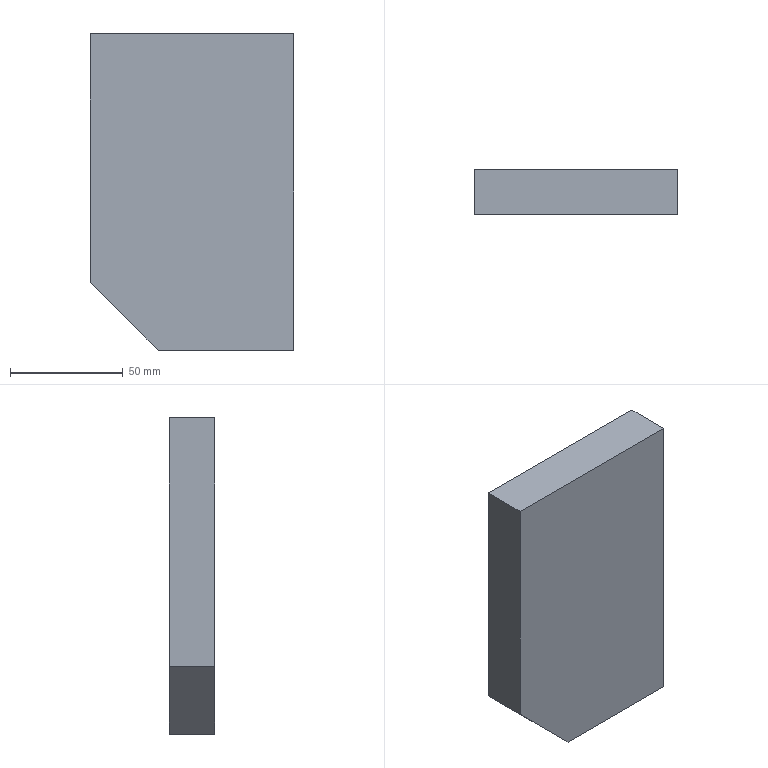Part | SolidWorks | features Extrusion 1 | 1 solid | 7 faces | box 90 x 20 x 140 mm | volume 243000 mm3 | plane 7
STEP:
#1=CARTESIAN_POINT('',(0.,0.,0.));
#2=VERTEX_POINT('',#1);
#3=CARTESIAN_POINT('',(0.,0.,-140.));
#4=VERTEX_POINT('',#3);
#5=CARTESIAN_POINT('',(0.,0.,0.));
#6=DIRECTION('',(0.,0.,-1.));
#7=VECTOR('',#6,1000.);
#8=LINE('',#5,#7);
#9=EDGE_CURVE('',#2,#4,#8,.T.);
#10=ORIENTED_EDGE('',*,*,#9,.T.);
#11=CARTESIAN_POINT('',(0.,20.,-140.));
#12=VERTEX_POINT('',#11);
#13=CARTESIAN_POINT('',(0.,20.,-140.));
#14=DIRECTION('',(0.,-1.,0.));
#15=VECTOR('',#14,1000.);
#16=LINE('',#13,#15);
#17=EDGE_CURVE('',#12,#4,#16,.T.);
#18=ORIENTED_EDGE('',*,*,#17,.F.);
#19=CARTESIAN_POINT('',(0.,20.,0.));
#20=VERTEX_POINT('',#19);
#21=CARTESIAN_POINT('',(0.,20.,0.));
#22=DIRECTION('',(0.,0.,-1.));
#23=VECTOR('',#22,1000.);
#24=LINE('',#21,#23);
#25=EDGE_CURVE('',#20,#12,#24,.T.);
#26=ORIENTED_EDGE('',*,*,#25,.F.);
#27=CARTESIAN_POINT('',(0.,20.,0.));
#28=DIRECTION('',(0.,-1.,0.));
#29=VECTOR('',#28,1000.);
#30=LINE('',#27,#29);
#31=EDGE_CURVE('',#20,#2,#30,.T.);
#32=ORIENTED_EDGE('',*,*,#31,.T.);
#33=EDGE_LOOP('',(#10,#18,#26,#32));
#34=FACE_OUTER_BOUND('',#33,.T.);
#35=CARTESIAN_POINT('',(0.,20.,0.));
#36=DIRECTION('',(-1.,0.,0.));
#37=DIRECTION('',(0.,0.,1.));
#38=AXIS2_PLACEMENT_3D('',#35,#36,#37);
#39=PLANE('',#38);
#40=ADVANCED_FACE('',(#34),#39,.F.);
#41=CARTESIAN_POINT('',(-60.,0.,-140.));
#42=VERTEX_POINT('',#41);
#43=CARTESIAN_POINT('',(0.,0.,-140.));
#44=DIRECTION('',(-1.,0.,0.));
#45=VECTOR('',#44,1000.);
#46=LINE('',#43,#45);
#47=EDGE_CURVE('',#4,#42,#46,.T.);
#48=ORIENTED_EDGE('',*,*,#47,.T.);
#49=CARTESIAN_POINT('',(-60.,20.,-140.));
#50=VERTEX_POINT('',#49);
#51=CARTESIAN_POINT('',(-60.,20.,-140.));
#52=DIRECTION('',(0.,-1.,0.));
#53=VECTOR('',#52,1000.);
#54=LINE('',#51,#53);
#55=EDGE_CURVE('',#50,#42,#54,.T.);
#56=ORIENTED_EDGE('',*,*,#55,.F.);
#57=CARTESIAN_POINT('',(0.,20.,-140.));
#58=DIRECTION('',(-1.,0.,0.));
#59=VECTOR('',#58,1000.);
#60=LINE('',#57,#59);
#61=EDGE_CURVE('',#12,#50,#60,.T.);
#62=ORIENTED_EDGE('',*,*,#61,.F.);
#63=ORIENTED_EDGE('',*,*,#17,.T.);
#64=EDGE_LOOP('',(#48,#56,#62,#63));
#65=FACE_OUTER_BOUND('',#64,.T.);
#66=CARTESIAN_POINT('',(0.,20.,-140.));
#67=DIRECTION('',(0.,0.,1.));
#68=DIRECTION('',(1.,0.,0.));
#69=AXIS2_PLACEMENT_3D('',#66,#67,#68);
#70=PLANE('',#69);
#71=ADVANCED_FACE('',(#65),#70,.F.);
#72=CARTESIAN_POINT('',(-90.,0.,-110.));
#73=VERTEX_POINT('',#72);
#74=CARTESIAN_POINT('',(-90.,0.,-110.));
#75=DIRECTION('',(-0.7071,0.,0.7071));
#76=VECTOR('',#75,1000.);
#77=LINE('',#74,#76);
#78=EDGE_CURVE('',#42,#73,#77,.T.);
#79=ORIENTED_EDGE('',*,*,#78,.T.);
#80=CARTESIAN_POINT('',(-90.,20.,-110.));
#81=VERTEX_POINT('',#80);
#82=CARTESIAN_POINT('',(-90.,20.,-110.));
#83=DIRECTION('',(0.,-1.,0.));
#84=VECTOR('',#83,1000.);
#85=LINE('',#82,#84);
#86=EDGE_CURVE('',#81,#73,#85,.T.);
#87=ORIENTED_EDGE('',*,*,#86,.F.);
#88=CARTESIAN_POINT('',(-90.,20.,-110.));
#89=DIRECTION('',(-0.7071,0.,0.7071));
#90=VECTOR('',#89,1000.);
#91=LINE('',#88,#90);
#92=EDGE_CURVE('',#50,#81,#91,.T.);
#93=ORIENTED_EDGE('',*,*,#92,.F.);
#94=ORIENTED_EDGE('',*,*,#55,.T.);
#95=EDGE_LOOP('',(#79,#87,#93,#94));
#96=FACE_OUTER_BOUND('',#95,.T.);
#97=CARTESIAN_POINT('',(-90.,20.,-110.));
#98=DIRECTION('',(0.7071,0.,0.7071));
#99=DIRECTION('',(0.7071,0.,-0.7071));
#100=AXIS2_PLACEMENT_3D('',#97,#98,#99);
#101=PLANE('',#100);
#102=ADVANCED_FACE('',(#96),#101,.F.);
#103=CARTESIAN_POINT('',(-90.,0.,0.));
#104=VERTEX_POINT('',#103);
#105=CARTESIAN_POINT('',(-90.,0.,0.));
#106=DIRECTION('',(0.,0.,1.));
#107=VECTOR('',#106,1000.);
#108=LINE('',#105,#107);
#109=EDGE_CURVE('',#73,#104,#108,.T.);
#110=ORIENTED_EDGE('',*,*,#109,.T.);
#111=CARTESIAN_POINT('',(-90.,20.,0.));
#112=VERTEX_POINT('',#111);
#113=CARTESIAN_POINT('',(-90.,20.,0.));
#114=DIRECTION('',(0.,-1.,0.));
#115=VECTOR('',#114,1000.);
#116=LINE('',#113,#115);
#117=EDGE_CURVE('',#112,#104,#116,.T.);
#118=ORIENTED_EDGE('',*,*,#117,.F.);
#119=CARTESIAN_POINT('',(-90.,20.,0.));
#120=DIRECTION('',(0.,0.,1.));
#121=VECTOR('',#120,1000.);
#122=LINE('',#119,#121);
#123=EDGE_CURVE('',#81,#112,#122,.T.);
#124=ORIENTED_EDGE('',*,*,#123,.F.);
#125=ORIENTED_EDGE('',*,*,#86,.T.);
#126=EDGE_LOOP('',(#110,#118,#124,#125));
#127=FACE_OUTER_BOUND('',#126,.T.);
#128=CARTESIAN_POINT('',(-90.,20.,0.));
#129=DIRECTION('',(1.,0.,0.));
#130=DIRECTION('',(0.,0.,-1.));
#131=AXIS2_PLACEMENT_3D('',#128,#129,#130);
#132=PLANE('',#131);
#133=ADVANCED_FACE('',(#127),#132,.F.);
#134=CARTESIAN_POINT('',(0.,0.,0.));
#135=DIRECTION('',(1.,0.,0.));
#136=VECTOR('',#135,1000.);
#137=LINE('',#134,#136);
#138=EDGE_CURVE('',#104,#2,#137,.T.);
#139=ORIENTED_EDGE('',*,*,#138,.T.);
#140=ORIENTED_EDGE('',*,*,#31,.F.);
#141=CARTESIAN_POINT('',(0.,20.,0.));
#142=DIRECTION('',(1.,0.,0.));
#143=VECTOR('',#142,1000.);
#144=LINE('',#141,#143);
#145=EDGE_CURVE('',#112,#20,#144,.T.);
#146=ORIENTED_EDGE('',*,*,#145,.F.);
#147=ORIENTED_EDGE('',*,*,#117,.T.);
#148=EDGE_LOOP('',(#139,#140,#146,#147));
#149=FACE_OUTER_BOUND('',#148,.T.);
#150=CARTESIAN_POINT('',(0.,20.,0.));
#151=DIRECTION('',(0.,0.,-1.));
#152=DIRECTION('',(-1.,0.,0.));
#153=AXIS2_PLACEMENT_3D('',#150,#151,#152);
#154=PLANE('',#153);
#155=ADVANCED_FACE('',(#149),#154,.F.);
#156=ORIENTED_EDGE('',*,*,#25,.T.);
#157=ORIENTED_EDGE('',*,*,#61,.T.);
#158=ORIENTED_EDGE('',*,*,#92,.T.);
#159=ORIENTED_EDGE('',*,*,#123,.T.);
#160=ORIENTED_EDGE('',*,*,#145,.T.);
#161=EDGE_LOOP('',(#156,#157,#158,#159,#160));
#162=FACE_OUTER_BOUND('',#161,.T.);
#163=CARTESIAN_POINT('',(0.,20.,0.));
#164=DIRECTION('',(0.,1.,0.));
#165=DIRECTION('',(0.,0.,1.));
#166=AXIS2_PLACEMENT_3D('',#163,#164,#165);
#167=PLANE('',#166);
#168=ADVANCED_FACE('',(#162),#167,.T.);
#169=ORIENTED_EDGE('',*,*,#9,.F.);
#170=ORIENTED_EDGE('',*,*,#138,.F.);
#171=ORIENTED_EDGE('',*,*,#109,.F.);
#172=ORIENTED_EDGE('',*,*,#78,.F.);
#173=ORIENTED_EDGE('',*,*,#47,.F.);
#174=EDGE_LOOP('',(#169,#170,#171,#172,#173));
#175=FACE_OUTER_BOUND('',#174,.T.);
#176=CARTESIAN_POINT('',(0.,0.,0.));
#177=DIRECTION('',(0.,1.,0.));
#178=DIRECTION('',(0.,0.,1.));
#179=AXIS2_PLACEMENT_3D('',#176,#177,#178);
#180=PLANE('',#179);
#181=ADVANCED_FACE('',(#175),#180,.F.);
#182=CLOSED_SHELL('',(#40,#71,#102,#133,#155,#168,#181));
#183=MANIFOLD_SOLID_BREP('',#182);
#184=CARTESIAN_POINT('',(0.,0.,0.));
#185=DIRECTION('',(0.,0.,1.));
#186=DIRECTION('',(1.,0.,0.));
#187=AXIS2_PLACEMENT_3D('',#184,#185,#186);
#188=(LENGTH_UNIT()NAMED_UNIT(*)SI_UNIT(.MILLI.,.METRE.));
#189=UNCERTAINTY_MEASURE_WITH_UNIT(LENGTH_MEASURE(0.00001),#188,'','');
#190=(NAMED_UNIT(*)PLANE_ANGLE_UNIT()SI_UNIT($,.RADIAN.));
#191=(NAMED_UNIT(*)SI_UNIT($,.STERADIAN.)SOLID_ANGLE_UNIT());
#192=(GEOMETRIC_REPRESENTATION_CONTEXT(3)GLOBAL_UNCERTAINTY_ASSIGNED_CONTEXT((#189))GLOBAL_UNIT_ASSIGNED_CONTEXT((#188,#190,#191))REPRESENTATION_CONTEXT('',''));
#193=ADVANCED_BREP_SHAPE_REPRESENTATION('',(#183,#187),#192);